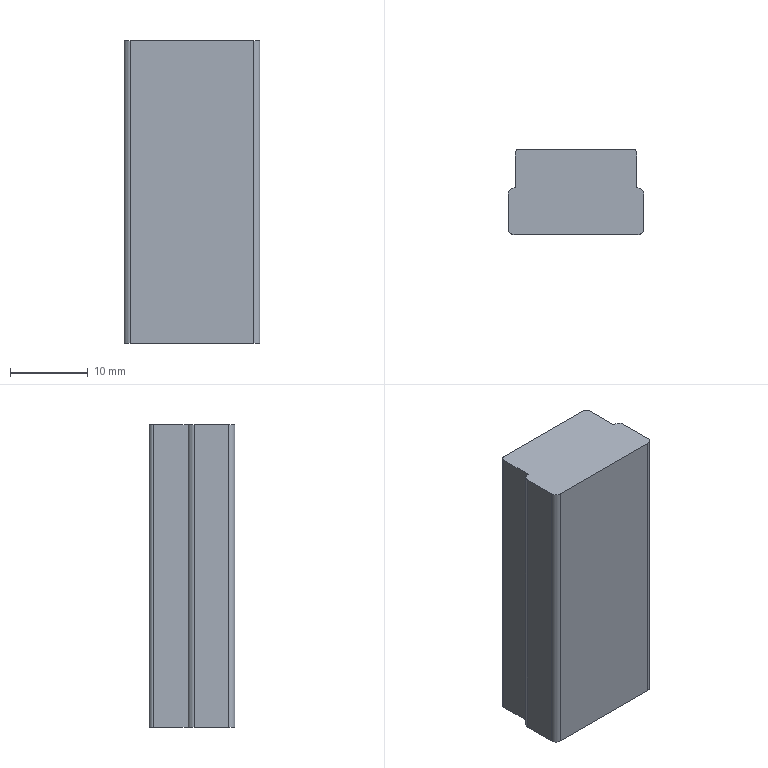Part | STEP file | LUOI GA PHIA DUOI | 1 solid | 16 faces | box 17.5 x 11 x 39 mm | volume 7111 mm3 | plane 10 | cylinder 6 | commonest cylinder face diameters 1.6 x4 1 x2
STEP:
#1=CARTESIAN_POINT('',(0.,0.,0.));
#2=DIRECTION('',(0.,0.,1.));
#3=DIRECTION('',(1.,0.,0.));
#4=AXIS2_PLACEMENT_3D('',#1,#2,#3);
#5=CARTESIAN_POINT('',(-16.7,0.,0.));
#6=VERTEX_POINT('',#5);
#7=CARTESIAN_POINT('',(-0.8,0.,0.));
#8=VERTEX_POINT('',#7);
#9=CARTESIAN_POINT('',(-0.8,0.,0.));
#10=DIRECTION('',(1.,0.,0.));
#11=VECTOR('',#10,1.);
#12=LINE('',#9,#11);
#13=CARTESIAN_POINT('',(-0.8,0.,0.));
#14=DIRECTION('',(0.,-1.,0.));
#15=DIRECTION('',(0.,0.,-1.));
#16=AXIS2_PLACEMENT_3D('',#13,#14,#15);
#17=PLANE('',#16);
#18=CARTESIAN_POINT('',(0.,0.));
#19=DIRECTION('',(0.,1.));
#20=VECTOR('',#19,1.);
#21=LINE('',#18,#20);
#22=(GEOMETRIC_REPRESENTATION_CONTEXT(2)PARAMETRIC_REPRESENTATION_CONTEXT()REPRESENTATION_CONTEXT('',''));
#23=DEFINITIONAL_REPRESENTATION('',(#21),#22);
#24=PCURVE('',#17,#23);
#25=CARTESIAN_POINT('',(-8.75,5.346,0.));
#26=DIRECTION('',(0.,0.,1.));
#27=DIRECTION('',(1.,0.,0.));
#28=AXIS2_PLACEMENT_3D('',#25,#26,#27);
#29=PLANE('',#28);
#30=CARTESIAN_POINT('',(7.95,-5.346));
#31=DIRECTION('',(1.,0.));
#32=VECTOR('',#31,1.);
#33=LINE('',#30,#32);
#34=(GEOMETRIC_REPRESENTATION_CONTEXT(2)PARAMETRIC_REPRESENTATION_CONTEXT()REPRESENTATION_CONTEXT('',''));
#35=DEFINITIONAL_REPRESENTATION('',(#33),#34);
#36=PCURVE('',#29,#35);
#37=SURFACE_CURVE('',#12,(#24,#36),.PCURVE_S1.);
#38=EDGE_CURVE('',#6,#8,#37,.T.);
#39=ORIENTED_EDGE('',*,*,#38,.T.);
#40=CARTESIAN_POINT('',(-0.8,0.,39.));
#41=VERTEX_POINT('',#40);
#42=CARTESIAN_POINT('',(-0.8,0.,0.));
#43=DIRECTION('',(0.,0.,1.));
#44=VECTOR('',#43,1.);
#45=LINE('',#42,#44);
#46=CARTESIAN_POINT('',(0.,0.));
#47=DIRECTION('',(-1.,0.));
#48=VECTOR('',#47,1.);
#49=LINE('',#46,#48);
#50=(GEOMETRIC_REPRESENTATION_CONTEXT(2)PARAMETRIC_REPRESENTATION_CONTEXT()REPRESENTATION_CONTEXT('',''));
#51=DEFINITIONAL_REPRESENTATION('',(#49),#50);
#52=PCURVE('',#17,#51);
#53=CARTESIAN_POINT('',(-0.8,0.8,0.));
#54=DIRECTION('',(0.,0.,1.));
#55=DIRECTION('',(1.,0.,0.));
#56=AXIS2_PLACEMENT_3D('',#53,#54,#55);
#57=CYLINDRICAL_SURFACE('',#56,0.8);
#58=CARTESIAN_POINT('',(4.712,0.));
#59=DIRECTION('',(0.,1.));
#60=VECTOR('',#59,1.);
#61=LINE('',#58,#60);
#62=(GEOMETRIC_REPRESENTATION_CONTEXT(2)PARAMETRIC_REPRESENTATION_CONTEXT()REPRESENTATION_CONTEXT('',''));
#63=DEFINITIONAL_REPRESENTATION('',(#61),#62);
#64=PCURVE('',#57,#63);
#65=SURFACE_CURVE('',#45,(#52,#64),.PCURVE_S1.);
#66=EDGE_CURVE('',#8,#41,#65,.T.);
#67=ORIENTED_EDGE('',*,*,#66,.T.);
#68=CARTESIAN_POINT('',(-16.7,0.,39.));
#69=VERTEX_POINT('',#68);
#70=CARTESIAN_POINT('',(-0.8,0.,39.));
#71=DIRECTION('',(-1.,0.,0.));
#72=VECTOR('',#71,1.);
#73=LINE('',#70,#72);
#74=CARTESIAN_POINT('',(-39.,0.));
#75=DIRECTION('',(0.,-1.));
#76=VECTOR('',#75,1.);
#77=LINE('',#74,#76);
#78=(GEOMETRIC_REPRESENTATION_CONTEXT(2)PARAMETRIC_REPRESENTATION_CONTEXT()REPRESENTATION_CONTEXT('',''));
#79=DEFINITIONAL_REPRESENTATION('',(#77),#78);
#80=PCURVE('',#17,#79);
#81=CARTESIAN_POINT('',(-8.75,5.346,39.));
#82=DIRECTION('',(0.,0.,1.));
#83=DIRECTION('',(1.,0.,0.));
#84=AXIS2_PLACEMENT_3D('',#81,#82,#83);
#85=PLANE('',#84);
#86=CARTESIAN_POINT('',(7.95,-5.346));
#87=DIRECTION('',(-1.,0.));
#88=VECTOR('',#87,1.);
#89=LINE('',#86,#88);
#90=(GEOMETRIC_REPRESENTATION_CONTEXT(2)PARAMETRIC_REPRESENTATION_CONTEXT()REPRESENTATION_CONTEXT('',''));
#91=DEFINITIONAL_REPRESENTATION('',(#89),#90);
#92=PCURVE('',#85,#91);
#93=SURFACE_CURVE('',#73,(#80,#92),.PCURVE_S1.);
#94=EDGE_CURVE('',#41,#69,#93,.T.);
#95=ORIENTED_EDGE('',*,*,#94,.T.);
#96=CARTESIAN_POINT('',(-16.7,0.,0.));
#97=DIRECTION('',(0.,0.,-1.));
#98=VECTOR('',#97,1.);
#99=LINE('',#96,#98);
#100=CARTESIAN_POINT('',(0.,-15.9));
#101=DIRECTION('',(1.,0.));
#102=VECTOR('',#101,1.);
#103=LINE('',#100,#102);
#104=(GEOMETRIC_REPRESENTATION_CONTEXT(2)PARAMETRIC_REPRESENTATION_CONTEXT()REPRESENTATION_CONTEXT('',''));
#105=DEFINITIONAL_REPRESENTATION('',(#103),#104);
#106=PCURVE('',#17,#105);
#107=CARTESIAN_POINT('',(-16.7,0.8,0.));
#108=DIRECTION('',(0.,0.,1.));
#109=DIRECTION('',(1.,0.,0.));
#110=AXIS2_PLACEMENT_3D('',#107,#108,#109);
#111=CYLINDRICAL_SURFACE('',#110,0.8);
#112=CARTESIAN_POINT('',(4.712,0.));
#113=DIRECTION('',(0.,-1.));
#114=VECTOR('',#113,1.);
#115=LINE('',#112,#114);
#116=(GEOMETRIC_REPRESENTATION_CONTEXT(2)PARAMETRIC_REPRESENTATION_CONTEXT()REPRESENTATION_CONTEXT('',''));
#117=DEFINITIONAL_REPRESENTATION('',(#115),#116);
#118=PCURVE('',#111,#117);
#119=SURFACE_CURVE('',#99,(#106,#118),.PCURVE_S1.);
#120=EDGE_CURVE('',#69,#6,#119,.T.);
#121=ORIENTED_EDGE('',*,*,#120,.T.);
#122=EDGE_LOOP('',(#39,#67,#95,#121));
#123=FACE_BOUND('',#122,.T.);
#124=ADVANCED_FACE('',(#123),#17,.T.);
#125=CARTESIAN_POINT('',(0.,0.8,0.));
#126=VERTEX_POINT('',#125);
#127=CARTESIAN_POINT('',(-0.8,0.8,0.));
#128=DIRECTION('',(0.,0.,1.));
#129=DIRECTION('',(1.,0.,0.));
#130=AXIS2_PLACEMENT_3D('',#127,#128,#129);
#131=CIRCLE('',#130,0.8);
#132=CARTESIAN_POINT('',(0.,0.));
#133=DIRECTION('',(1.,0.));
#134=VECTOR('',#133,1.);
#135=LINE('',#132,#134);
#136=(GEOMETRIC_REPRESENTATION_CONTEXT(2)PARAMETRIC_REPRESENTATION_CONTEXT()REPRESENTATION_CONTEXT('',''));
#137=DEFINITIONAL_REPRESENTATION('',(#135),#136);
#138=PCURVE('',#57,#137);
#139=CARTESIAN_POINT('',(7.95,-4.546));
#140=DIRECTION('',(1.,0.));
#141=AXIS2_PLACEMENT_2D('',#139,#140);
#142=CIRCLE('',#141,0.8);
#143=(GEOMETRIC_REPRESENTATION_CONTEXT(2)PARAMETRIC_REPRESENTATION_CONTEXT()REPRESENTATION_CONTEXT('',''));
#144=DEFINITIONAL_REPRESENTATION('',(#142),#143);
#145=PCURVE('',#29,#144);
#146=SURFACE_CURVE('',#131,(#138,#145),.PCURVE_S1.);
#147=EDGE_CURVE('',#8,#126,#146,.T.);
#148=ORIENTED_EDGE('',*,*,#147,.T.);
#149=CARTESIAN_POINT('',(0.,0.8,39.));
#150=VERTEX_POINT('',#149);
#151=CARTESIAN_POINT('',(0.,0.8,0.));
#152=DIRECTION('',(0.,0.,1.));
#153=VECTOR('',#152,1.);
#154=LINE('',#151,#153);
#155=CARTESIAN_POINT('',(6.283,0.));
#156=DIRECTION('',(0.,1.));
#157=VECTOR('',#156,1.);
#158=LINE('',#155,#157);
#159=(GEOMETRIC_REPRESENTATION_CONTEXT(2)PARAMETRIC_REPRESENTATION_CONTEXT()REPRESENTATION_CONTEXT('',''));
#160=DEFINITIONAL_REPRESENTATION('',(#158),#159);
#161=PCURVE('',#57,#160);
#162=CARTESIAN_POINT('',(0.,5.2,0.));
#163=DIRECTION('',(1.,0.,0.));
#164=DIRECTION('',(0.,0.,-1.));
#165=AXIS2_PLACEMENT_3D('',#162,#163,#164);
#166=PLANE('',#165);
#167=CARTESIAN_POINT('',(0.,-4.4));
#168=DIRECTION('',(-1.,0.));
#169=VECTOR('',#168,1.);
#170=LINE('',#167,#169);
#171=(GEOMETRIC_REPRESENTATION_CONTEXT(2)PARAMETRIC_REPRESENTATION_CONTEXT()REPRESENTATION_CONTEXT('',''));
#172=DEFINITIONAL_REPRESENTATION('',(#170),#171);
#173=PCURVE('',#166,#172);
#174=SURFACE_CURVE('',#154,(#161,#173),.PCURVE_S1.);
#175=EDGE_CURVE('',#126,#150,#174,.T.);
#176=ORIENTED_EDGE('',*,*,#175,.T.);
#177=CARTESIAN_POINT('',(-0.8,0.8,39.));
#178=DIRECTION('',(0.,0.,-1.));
#179=DIRECTION('',(1.,0.,0.));
#180=AXIS2_PLACEMENT_3D('',#177,#178,#179);
#181=CIRCLE('',#180,0.8);
#182=CARTESIAN_POINT('',(6.283,39.));
#183=DIRECTION('',(-1.,0.));
#184=VECTOR('',#183,1.);
#185=LINE('',#182,#184);
#186=(GEOMETRIC_REPRESENTATION_CONTEXT(2)PARAMETRIC_REPRESENTATION_CONTEXT()REPRESENTATION_CONTEXT('',''));
#187=DEFINITIONAL_REPRESENTATION('',(#185),#186);
#188=PCURVE('',#57,#187);
#189=CARTESIAN_POINT('',(8.75,-4.546));
#190=CARTESIAN_POINT('',(8.75,-5.932));
#191=CARTESIAN_POINT('',(7.55,-5.239));
#192=CARTESIAN_POINT('',(6.35,-4.546));
#193=CARTESIAN_POINT('',(7.55,-3.854));
#194=CARTESIAN_POINT('',(8.75,-3.161));
#195=CARTESIAN_POINT('',(8.75,-4.546));
#196=(BOUNDED_CURVE()B_SPLINE_CURVE(2,(#189,#190,#191,#192,#193,#194,#195),.UNSPECIFIED.,.T.,.F.)B_SPLINE_CURVE_WITH_KNOTS((1,2,2,2,2,1),(-2.094,0.,2.094,4.189,6.283,8.378),.UNSPECIFIED.)CURVE()GEOMETRIC_REPRESENTATION_ITEM()RATIONAL_B_SPLINE_CURVE((1.,0.5,1.,0.5,1.,0.5,1.))REPRESENTATION_ITEM(''));
#197=(GEOMETRIC_REPRESENTATION_CONTEXT(2)PARAMETRIC_REPRESENTATION_CONTEXT()REPRESENTATION_CONTEXT('',''));
#198=DEFINITIONAL_REPRESENTATION('',(#196),#197);
#199=PCURVE('',#85,#198);
#200=SURFACE_CURVE('',#181,(#188,#199),.PCURVE_S1.);
#201=EDGE_CURVE('',#150,#41,#200,.T.);
#202=ORIENTED_EDGE('',*,*,#201,.T.);
#203=ORIENTED_EDGE('',*,*,#66,.F.);
#204=EDGE_LOOP('',(#148,#176,#202,#203));
#205=FACE_BOUND('',#204,.T.);
#206=ADVANCED_FACE('',(#205),#57,.T.);
#207=CARTESIAN_POINT('',(-0.8,6.,0.));
#208=VERTEX_POINT('',#207);
#209=CARTESIAN_POINT('',(-0.95,6.,0.));
#210=VERTEX_POINT('',#209);
#211=CARTESIAN_POINT('',(-0.95,6.,0.));
#212=DIRECTION('',(-1.,0.,0.));
#213=VECTOR('',#212,1.);
#214=LINE('',#211,#213);
#215=CARTESIAN_POINT('',(7.8,0.6535));
#216=DIRECTION('',(-1.,0.));
#217=VECTOR('',#216,1.);
#218=LINE('',#215,#217);
#219=(GEOMETRIC_REPRESENTATION_CONTEXT(2)PARAMETRIC_REPRESENTATION_CONTEXT()REPRESENTATION_CONTEXT('',''));
#220=DEFINITIONAL_REPRESENTATION('',(#218),#219);
#221=PCURVE('',#29,#220);
#222=CARTESIAN_POINT('',(-0.95,6.,0.));
#223=DIRECTION('',(0.,1.,0.));
#224=DIRECTION('',(0.,0.,1.));
#225=AXIS2_PLACEMENT_3D('',#222,#223,#224);
#226=PLANE('',#225);
#227=CARTESIAN_POINT('',(0.,0.));
#228=DIRECTION('',(0.,-1.));
#229=VECTOR('',#228,1.);
#230=LINE('',#227,#229);
#231=(GEOMETRIC_REPRESENTATION_CONTEXT(2)PARAMETRIC_REPRESENTATION_CONTEXT()REPRESENTATION_CONTEXT('',''));
#232=DEFINITIONAL_REPRESENTATION('',(#230),#231);
#233=PCURVE('',#226,#232);
#234=SURFACE_CURVE('',#214,(#221,#233),.PCURVE_S1.);
#235=EDGE_CURVE('',#208,#210,#234,.T.);
#236=ORIENTED_EDGE('',*,*,#235,.F.);
#237=CARTESIAN_POINT('',(0.,5.2,0.));
#238=VERTEX_POINT('',#237);
#239=CARTESIAN_POINT('',(-0.8,5.2,0.));
#240=DIRECTION('',(0.,0.,1.));
#241=DIRECTION('',(1.,0.,0.));
#242=AXIS2_PLACEMENT_3D('',#239,#240,#241);
#243=CIRCLE('',#242,0.8);
#244=CARTESIAN_POINT('',(7.95,-0.1465));
#245=DIRECTION('',(1.,0.));
#246=AXIS2_PLACEMENT_2D('',#244,#245);
#247=CIRCLE('',#246,0.8);
#248=(GEOMETRIC_REPRESENTATION_CONTEXT(2)PARAMETRIC_REPRESENTATION_CONTEXT()REPRESENTATION_CONTEXT('',''));
#249=DEFINITIONAL_REPRESENTATION('',(#247),#248);
#250=PCURVE('',#29,#249);
#251=CARTESIAN_POINT('',(-0.8,5.2,0.));
#252=DIRECTION('',(0.,0.,1.));
#253=DIRECTION('',(1.,0.,0.));
#254=AXIS2_PLACEMENT_3D('',#251,#252,#253);
#255=CYLINDRICAL_SURFACE('',#254,0.8);
#256=CARTESIAN_POINT('',(0.,0.));
#257=DIRECTION('',(1.,0.));
#258=VECTOR('',#257,1.);
#259=LINE('',#256,#258);
#260=(GEOMETRIC_REPRESENTATION_CONTEXT(2)PARAMETRIC_REPRESENTATION_CONTEXT()REPRESENTATION_CONTEXT('',''));
#261=DEFINITIONAL_REPRESENTATION('',(#259),#260);
#262=PCURVE('',#255,#261);
#263=SURFACE_CURVE('',#243,(#250,#262),.PCURVE_S1.);
#264=EDGE_CURVE('',#238,#208,#263,.T.);
#265=ORIENTED_EDGE('',*,*,#264,.F.);
#266=CARTESIAN_POINT('',(0.,5.346,0.));
#267=DIRECTION('',(0.,1.,0.));
#268=VECTOR('',#267,1.);
#269=LINE('',#266,#268);
#270=CARTESIAN_POINT('',(8.75,0.));
#271=DIRECTION('',(0.,1.));
#272=VECTOR('',#271,1.);
#273=LINE('',#270,#272);
#274=(GEOMETRIC_REPRESENTATION_CONTEXT(2)PARAMETRIC_REPRESENTATION_CONTEXT()REPRESENTATION_CONTEXT('',''));
#275=DEFINITIONAL_REPRESENTATION('',(#273),#274);
#276=PCURVE('',#29,#275);
#277=CARTESIAN_POINT('',(0.,0.1465));
#278=DIRECTION('',(0.,1.));
#279=VECTOR('',#278,1.);
#280=LINE('',#277,#279);
#281=(GEOMETRIC_REPRESENTATION_CONTEXT(2)PARAMETRIC_REPRESENTATION_CONTEXT()REPRESENTATION_CONTEXT('',''));
#282=DEFINITIONAL_REPRESENTATION('',(#280),#281);
#283=PCURVE('',#166,#282);
#284=SURFACE_CURVE('',#269,(#276,#283),.PCURVE_S1.);
#285=EDGE_CURVE('',#126,#238,#284,.T.);
#286=ORIENTED_EDGE('',*,*,#285,.F.);
#287=ORIENTED_EDGE('',*,*,#147,.F.);
#288=ORIENTED_EDGE('',*,*,#38,.F.);
#289=CARTESIAN_POINT('',(-17.5,0.8,0.));
#290=VERTEX_POINT('',#289);
#291=CARTESIAN_POINT('',(-16.7,0.8,0.));
#292=DIRECTION('',(0.,0.,1.));
#293=DIRECTION('',(1.,0.,0.));
#294=AXIS2_PLACEMENT_3D('',#291,#292,#293);
#295=CIRCLE('',#294,0.8);
#296=CARTESIAN_POINT('',(-7.95,-4.546));
#297=DIRECTION('',(1.,0.));
#298=AXIS2_PLACEMENT_2D('',#296,#297);
#299=CIRCLE('',#298,0.8);
#300=(GEOMETRIC_REPRESENTATION_CONTEXT(2)PARAMETRIC_REPRESENTATION_CONTEXT()REPRESENTATION_CONTEXT('',''));
#301=DEFINITIONAL_REPRESENTATION('',(#299),#300);
#302=PCURVE('',#29,#301);
#303=CARTESIAN_POINT('',(0.,0.));
#304=DIRECTION('',(1.,0.));
#305=VECTOR('',#304,1.);
#306=LINE('',#303,#305);
#307=(GEOMETRIC_REPRESENTATION_CONTEXT(2)PARAMETRIC_REPRESENTATION_CONTEXT()REPRESENTATION_CONTEXT('',''));
#308=DEFINITIONAL_REPRESENTATION('',(#306),#307);
#309=PCURVE('',#111,#308);
#310=SURFACE_CURVE('',#295,(#302,#309),.PCURVE_S1.);
#311=EDGE_CURVE('',#290,#6,#310,.T.);
#312=ORIENTED_EDGE('',*,*,#311,.F.);
#313=CARTESIAN_POINT('',(-17.5,5.2,0.));
#314=VERTEX_POINT('',#313);
#315=CARTESIAN_POINT('',(-17.5,5.346,0.));
#316=DIRECTION('',(0.,-1.,0.));
#317=VECTOR('',#316,1.);
#318=LINE('',#315,#317);
#319=CARTESIAN_POINT('',(-8.75,0.));
#320=DIRECTION('',(0.,-1.));
#321=VECTOR('',#320,1.);
#322=LINE('',#319,#321);
#323=(GEOMETRIC_REPRESENTATION_CONTEXT(2)PARAMETRIC_REPRESENTATION_CONTEXT()REPRESENTATION_CONTEXT('',''));
#324=DEFINITIONAL_REPRESENTATION('',(#322),#323);
#325=PCURVE('',#29,#324);
#326=CARTESIAN_POINT('',(-17.5,0.8,0.));
#327=DIRECTION('',(-1.,0.,0.));
#328=DIRECTION('',(0.,0.,1.));
#329=AXIS2_PLACEMENT_3D('',#326,#327,#328);
#330=PLANE('',#329);
#331=CARTESIAN_POINT('',(0.,4.546));
#332=DIRECTION('',(0.,-1.));
#333=VECTOR('',#332,1.);
#334=LINE('',#331,#333);
#335=(GEOMETRIC_REPRESENTATION_CONTEXT(2)PARAMETRIC_REPRESENTATION_CONTEXT()REPRESENTATION_CONTEXT('',''));
#336=DEFINITIONAL_REPRESENTATION('',(#334),#335);
#337=PCURVE('',#330,#336);
#338=SURFACE_CURVE('',#318,(#325,#337),.PCURVE_S1.);
#339=EDGE_CURVE('',#314,#290,#338,.T.);
#340=ORIENTED_EDGE('',*,*,#339,.F.);
#341=CARTESIAN_POINT('',(-16.7,6.,0.));
#342=VERTEX_POINT('',#341);
#343=CARTESIAN_POINT('',(-16.7,5.2,0.));
#344=DIRECTION('',(0.,0.,1.));
#345=DIRECTION('',(1.,0.,0.));
#346=AXIS2_PLACEMENT_3D('',#343,#344,#345);
#347=CIRCLE('',#346,0.8);
#348=CARTESIAN_POINT('',(-7.95,-0.1465));
#349=DIRECTION('',(1.,0.));
#350=AXIS2_PLACEMENT_2D('',#348,#349);
#351=CIRCLE('',#350,0.8);
#352=(GEOMETRIC_REPRESENTATION_CONTEXT(2)PARAMETRIC_REPRESENTATION_CONTEXT()REPRESENTATION_CONTEXT('',''));
#353=DEFINITIONAL_REPRESENTATION('',(#351),#352);
#354=PCURVE('',#29,#353);
#355=CARTESIAN_POINT('',(-16.7,5.2,0.));
#356=DIRECTION('',(0.,0.,1.));
#357=DIRECTION('',(1.,0.,0.));
#358=AXIS2_PLACEMENT_3D('',#355,#356,#357);
#359=CYLINDRICAL_SURFACE('',#358,0.8);
#360=CARTESIAN_POINT('',(0.,0.));
#361=DIRECTION('',(1.,0.));
#362=VECTOR('',#361,1.);
#363=LINE('',#360,#362);
#364=(GEOMETRIC_REPRESENTATION_CONTEXT(2)PARAMETRIC_REPRESENTATION_CONTEXT()REPRESENTATION_CONTEXT('',''));
#365=DEFINITIONAL_REPRESENTATION('',(#363),#364);
#366=PCURVE('',#359,#365);
#367=SURFACE_CURVE('',#347,(#354,#366),.PCURVE_S1.);
#368=EDGE_CURVE('',#342,#314,#367,.T.);
#369=ORIENTED_EDGE('',*,*,#368,.F.);
#370=CARTESIAN_POINT('',(-16.55,6.,0.));
#371=VERTEX_POINT('',#370);
#372=CARTESIAN_POINT('',(-16.7,6.,0.));
#373=DIRECTION('',(-1.,0.,0.));
#374=VECTOR('',#373,1.);
#375=LINE('',#372,#374);
#376=CARTESIAN_POINT('',(-7.95,0.6535));
#377=DIRECTION('',(-1.,0.));
#378=VECTOR('',#377,1.);
#379=LINE('',#376,#378);
#380=(GEOMETRIC_REPRESENTATION_CONTEXT(2)PARAMETRIC_REPRESENTATION_CONTEXT()REPRESENTATION_CONTEXT('',''));
#381=DEFINITIONAL_REPRESENTATION('',(#379),#380);
#382=PCURVE('',#29,#381);
#383=CARTESIAN_POINT('',(-16.7,6.,0.));
#384=DIRECTION('',(0.,1.,0.));
#385=DIRECTION('',(0.,0.,1.));
#386=AXIS2_PLACEMENT_3D('',#383,#384,#385);
#387=PLANE('',#386);
#388=CARTESIAN_POINT('',(0.,0.));
#389=DIRECTION('',(0.,-1.));
#390=VECTOR('',#389,1.);
#391=LINE('',#388,#390);
#392=(GEOMETRIC_REPRESENTATION_CONTEXT(2)PARAMETRIC_REPRESENTATION_CONTEXT()REPRESENTATION_CONTEXT('',''));
#393=DEFINITIONAL_REPRESENTATION('',(#391),#392);
#394=PCURVE('',#387,#393);
#395=SURFACE_CURVE('',#375,(#382,#394),.PCURVE_S1.);
#396=EDGE_CURVE('',#371,#342,#395,.T.);
#397=ORIENTED_EDGE('',*,*,#396,.F.);
#398=CARTESIAN_POINT('',(-16.55,10.5,0.));
#399=VERTEX_POINT('',#398);
#400=CARTESIAN_POINT('',(-16.55,5.346,0.));
#401=DIRECTION('',(0.,-1.,0.));
#402=VECTOR('',#401,1.);
#403=LINE('',#400,#402);
#404=CARTESIAN_POINT('',(-7.8,0.));
#405=DIRECTION('',(0.,-1.));
#406=VECTOR('',#405,1.);
#407=LINE('',#404,#406);
#408=(GEOMETRIC_REPRESENTATION_CONTEXT(2)PARAMETRIC_REPRESENTATION_CONTEXT()REPRESENTATION_CONTEXT('',''));
#409=DEFINITIONAL_REPRESENTATION('',(#407),#408);
#410=PCURVE('',#29,#409);
#411=CARTESIAN_POINT('',(-16.55,6.,0.));
#412=DIRECTION('',(-1.,0.,0.));
#413=DIRECTION('',(0.,0.,1.));
#414=AXIS2_PLACEMENT_3D('',#411,#412,#413);
#415=PLANE('',#414);
#416=CARTESIAN_POINT('',(0.,-0.6535));
#417=DIRECTION('',(0.,-1.));
#418=VECTOR('',#417,1.);
#419=LINE('',#416,#418);
#420=(GEOMETRIC_REPRESENTATION_CONTEXT(2)PARAMETRIC_REPRESENTATION_CONTEXT()REPRESENTATION_CONTEXT('',''));
#421=DEFINITIONAL_REPRESENTATION('',(#419),#420);
#422=PCURVE('',#415,#421);
#423=SURFACE_CURVE('',#403,(#410,#422),.PCURVE_S1.);
#424=EDGE_CURVE('',#399,#371,#423,.T.);
#425=ORIENTED_EDGE('',*,*,#424,.F.);
#426=CARTESIAN_POINT('',(-16.05,11.,0.));
#427=VERTEX_POINT('',#426);
#428=CARTESIAN_POINT('',(-16.05,10.5,0.));
#429=DIRECTION('',(0.,0.,1.));
#430=DIRECTION('',(1.,0.,0.));
#431=AXIS2_PLACEMENT_3D('',#428,#429,#430);
#432=CIRCLE('',#431,0.5);
#433=CARTESIAN_POINT('',(-7.3,5.154));
#434=DIRECTION('',(1.,0.));
#435=AXIS2_PLACEMENT_2D('',#433,#434);
#436=CIRCLE('',#435,0.5);
#437=(GEOMETRIC_REPRESENTATION_CONTEXT(2)PARAMETRIC_REPRESENTATION_CONTEXT()REPRESENTATION_CONTEXT('',''));
#438=DEFINITIONAL_REPRESENTATION('',(#436),#437);
#439=PCURVE('',#29,#438);
#440=CARTESIAN_POINT('',(-16.05,10.5,0.));
#441=DIRECTION('',(0.,0.,1.));
#442=DIRECTION('',(1.,0.,0.));
#443=AXIS2_PLACEMENT_3D('',#440,#441,#442);
#444=CYLINDRICAL_SURFACE('',#443,0.5);
#445=CARTESIAN_POINT('',(0.,0.));
#446=DIRECTION('',(1.,0.));
#447=VECTOR('',#446,1.);
#448=LINE('',#445,#447);
#449=(GEOMETRIC_REPRESENTATION_CONTEXT(2)PARAMETRIC_REPRESENTATION_CONTEXT()REPRESENTATION_CONTEXT('',''));
#450=DEFINITIONAL_REPRESENTATION('',(#448),#449);
#451=PCURVE('',#444,#450);
#452=SURFACE_CURVE('',#432,(#439,#451),.PCURVE_S1.);
#453=EDGE_CURVE('',#427,#399,#452,.T.);
#454=ORIENTED_EDGE('',*,*,#453,.F.);
#455=CARTESIAN_POINT('',(-1.45,11.,0.));
#456=VERTEX_POINT('',#455);
#457=CARTESIAN_POINT('',(-8.75,11.,0.));
#458=DIRECTION('',(-1.,0.,0.));
#459=VECTOR('',#458,1.);
#460=LINE('',#457,#459);
#461=CARTESIAN_POINT('',(0.,5.654));
#462=DIRECTION('',(-1.,0.));
#463=VECTOR('',#462,1.);
#464=LINE('',#461,#463);
#465=(GEOMETRIC_REPRESENTATION_CONTEXT(2)PARAMETRIC_REPRESENTATION_CONTEXT()REPRESENTATION_CONTEXT('',''));
#466=DEFINITIONAL_REPRESENTATION('',(#464),#465);
#467=PCURVE('',#29,#466);
#468=CARTESIAN_POINT('',(-16.05,11.,0.));
#469=DIRECTION('',(0.,1.,0.));
#470=DIRECTION('',(0.,0.,1.));
#471=AXIS2_PLACEMENT_3D('',#468,#469,#470);
#472=PLANE('',#471);
#473=CARTESIAN_POINT('',(0.,7.3));
#474=DIRECTION('',(0.,-1.));
#475=VECTOR('',#474,1.);
#476=LINE('',#473,#475);
#477=(GEOMETRIC_REPRESENTATION_CONTEXT(2)PARAMETRIC_REPRESENTATION_CONTEXT()REPRESENTATION_CONTEXT('',''));
#478=DEFINITIONAL_REPRESENTATION('',(#476),#477);
#479=PCURVE('',#472,#478);
#480=SURFACE_CURVE('',#460,(#467,#479),.PCURVE_S1.);
#481=EDGE_CURVE('',#456,#427,#480,.T.);
#482=ORIENTED_EDGE('',*,*,#481,.F.);
#483=CARTESIAN_POINT('',(-0.95,10.5,0.));
#484=VERTEX_POINT('',#483);
#485=CARTESIAN_POINT('',(-1.45,10.5,0.));
#486=DIRECTION('',(0.,0.,1.));
#487=DIRECTION('',(1.,0.,0.));
#488=AXIS2_PLACEMENT_3D('',#485,#486,#487);
#489=CIRCLE('',#488,0.5);
#490=CARTESIAN_POINT('',(7.3,5.154));
#491=DIRECTION('',(1.,0.));
#492=AXIS2_PLACEMENT_2D('',#490,#491);
#493=CIRCLE('',#492,0.5);
#494=(GEOMETRIC_REPRESENTATION_CONTEXT(2)PARAMETRIC_REPRESENTATION_CONTEXT()REPRESENTATION_CONTEXT('',''));
#495=DEFINITIONAL_REPRESENTATION('',(#493),#494);
#496=PCURVE('',#29,#495);
#497=CARTESIAN_POINT('',(-1.45,10.5,0.));
#498=DIRECTION('',(0.,0.,1.));
#499=DIRECTION('',(1.,0.,0.));
#500=AXIS2_PLACEMENT_3D('',#497,#498,#499);
#501=CYLINDRICAL_SURFACE('',#500,0.5);
#502=CARTESIAN_POINT('',(0.,0.));
#503=DIRECTION('',(1.,0.));
#504=VECTOR('',#503,1.);
#505=LINE('',#502,#504);
#506=(GEOMETRIC_REPRESENTATION_CONTEXT(2)PARAMETRIC_REPRESENTATION_CONTEXT()REPRESENTATION_CONTEXT('',''));
#507=DEFINITIONAL_REPRESENTATION('',(#505),#506);
#508=PCURVE('',#501,#507);
#509=SURFACE_CURVE('',#489,(#496,#508),.PCURVE_S1.);
#510=EDGE_CURVE('',#484,#456,#509,.T.);
#511=ORIENTED_EDGE('',*,*,#510,.F.);
#512=CARTESIAN_POINT('',(-0.95,5.346,0.));
#513=DIRECTION('',(0.,1.,0.));
#514=VECTOR('',#513,1.);
#515=LINE('',#512,#514);
#516=CARTESIAN_POINT('',(7.8,0.));
#517=DIRECTION('',(0.,1.));
#518=VECTOR('',#517,1.);
#519=LINE('',#516,#518);
#520=(GEOMETRIC_REPRESENTATION_CONTEXT(2)PARAMETRIC_REPRESENTATION_CONTEXT()REPRESENTATION_CONTEXT('',''));
#521=DEFINITIONAL_REPRESENTATION('',(#519),#520);
#522=PCURVE('',#29,#521);
#523=CARTESIAN_POINT('',(-0.95,10.5,0.));
#524=DIRECTION('',(1.,0.,0.));
#525=DIRECTION('',(0.,0.,-1.));
#526=AXIS2_PLACEMENT_3D('',#523,#524,#525);
#527=PLANE('',#526);
#528=CARTESIAN_POINT('',(0.,-5.154));
#529=DIRECTION('',(0.,1.));
#530=VECTOR('',#529,1.);
#531=LINE('',#528,#530);
#532=(GEOMETRIC_REPRESENTATION_CONTEXT(2)PARAMETRIC_REPRESENTATION_CONTEXT()REPRESENTATION_CONTEXT('',''));
#533=DEFINITIONAL_REPRESENTATION('',(#531),#532);
#534=PCURVE('',#527,#533);
#535=SURFACE_CURVE('',#515,(#522,#534),.PCURVE_S1.);
#536=EDGE_CURVE('',#210,#484,#535,.T.);
#537=ORIENTED_EDGE('',*,*,#536,.F.);
#538=EDGE_LOOP('',(#236,#265,#286,#287,#288,#312,#340,#369,#397,#425,#454,#482,#511,#537));
#539=FACE_BOUND('',#538,.T.);
#540=ADVANCED_FACE('',(#539),#29,.F.);
#541=ORIENTED_EDGE('',*,*,#311,.T.);
#542=ORIENTED_EDGE('',*,*,#120,.F.);
#543=CARTESIAN_POINT('',(-17.5,0.8,39.));
#544=VERTEX_POINT('',#543);
#545=CARTESIAN_POINT('',(-16.7,0.8,39.));
#546=DIRECTION('',(0.,0.,-1.));
#547=DIRECTION('',(1.,0.,0.));
#548=AXIS2_PLACEMENT_3D('',#545,#546,#547);
#549=CIRCLE('',#548,0.8);
#550=CARTESIAN_POINT('',(6.283,39.));
#551=DIRECTION('',(-1.,0.));
#552=VECTOR('',#551,1.);
#553=LINE('',#550,#552);
#554=(GEOMETRIC_REPRESENTATION_CONTEXT(2)PARAMETRIC_REPRESENTATION_CONTEXT()REPRESENTATION_CONTEXT('',''));
#555=DEFINITIONAL_REPRESENTATION('',(#553),#554);
#556=PCURVE('',#111,#555);
#557=CARTESIAN_POINT('',(-7.15,-4.546));
#558=CARTESIAN_POINT('',(-7.15,-5.932));
#559=CARTESIAN_POINT('',(-8.35,-5.239));
#560=CARTESIAN_POINT('',(-9.55,-4.546));
#561=CARTESIAN_POINT('',(-8.35,-3.854));
#562=CARTESIAN_POINT('',(-7.15,-3.161));
#563=CARTESIAN_POINT('',(-7.15,-4.546));
#564=(BOUNDED_CURVE()B_SPLINE_CURVE(2,(#557,#558,#559,#560,#561,#562,#563),.UNSPECIFIED.,.T.,.F.)B_SPLINE_CURVE_WITH_KNOTS((1,2,2,2,2,1),(-2.094,0.,2.094,4.189,6.283,8.378),.UNSPECIFIED.)CURVE()GEOMETRIC_REPRESENTATION_ITEM()RATIONAL_B_SPLINE_CURVE((1.,0.5,1.,0.5,1.,0.5,1.))REPRESENTATION_ITEM(''));
#565=(GEOMETRIC_REPRESENTATION_CONTEXT(2)PARAMETRIC_REPRESENTATION_CONTEXT()REPRESENTATION_CONTEXT('',''));
#566=DEFINITIONAL_REPRESENTATION('',(#564),#565);
#567=PCURVE('',#85,#566);
#568=SURFACE_CURVE('',#549,(#556,#567),.PCURVE_S1.);
#569=EDGE_CURVE('',#69,#544,#568,.T.);
#570=ORIENTED_EDGE('',*,*,#569,.T.);
#571=CARTESIAN_POINT('',(-17.5,0.8,0.));
#572=DIRECTION('',(0.,0.,-1.));
#573=VECTOR('',#572,1.);
#574=LINE('',#571,#573);
#575=CARTESIAN_POINT('',(3.142,0.));
#576=DIRECTION('',(0.,-1.));
#577=VECTOR('',#576,1.);
#578=LINE('',#575,#577);
#579=(GEOMETRIC_REPRESENTATION_CONTEXT(2)PARAMETRIC_REPRESENTATION_CONTEXT()REPRESENTATION_CONTEXT('',''));
#580=DEFINITIONAL_REPRESENTATION('',(#578),#579);
#581=PCURVE('',#111,#580);
#582=CARTESIAN_POINT('',(0.,0.));
#583=DIRECTION('',(-1.,0.));
#584=VECTOR('',#583,1.);
#585=LINE('',#582,#584);
#586=(GEOMETRIC_REPRESENTATION_CONTEXT(2)PARAMETRIC_REPRESENTATION_CONTEXT()REPRESENTATION_CONTEXT('',''));
#587=DEFINITIONAL_REPRESENTATION('',(#585),#586);
#588=PCURVE('',#330,#587);
#589=SURFACE_CURVE('',#574,(#581,#588),.PCURVE_S1.);
#590=EDGE_CURVE('',#544,#290,#589,.T.);
#591=ORIENTED_EDGE('',*,*,#590,.T.);
#592=EDGE_LOOP('',(#541,#542,#570,#591));
#593=FACE_BOUND('',#592,.T.);
#594=ADVANCED_FACE('',(#593),#111,.T.);
#595=CARTESIAN_POINT('',(0.,5.2,39.));
#596=VERTEX_POINT('',#595);
#597=CARTESIAN_POINT('',(0.,5.346,39.));
#598=DIRECTION('',(0.,1.,0.));
#599=VECTOR('',#598,1.);
#600=LINE('',#597,#599);
#601=CARTESIAN_POINT('',(8.75,0.));
#602=DIRECTION('',(0.,1.));
#603=VECTOR('',#602,1.);
#604=LINE('',#601,#603);
#605=(GEOMETRIC_REPRESENTATION_CONTEXT(2)PARAMETRIC_REPRESENTATION_CONTEXT()REPRESENTATION_CONTEXT('',''));
#606=DEFINITIONAL_REPRESENTATION('',(#604),#605);
#607=PCURVE('',#85,#606);
#608=CARTESIAN_POINT('',(-39.,0.1465));
#609=DIRECTION('',(0.,1.));
#610=VECTOR('',#609,1.);
#611=LINE('',#608,#610);
#612=(GEOMETRIC_REPRESENTATION_CONTEXT(2)PARAMETRIC_REPRESENTATION_CONTEXT()REPRESENTATION_CONTEXT('',''));
#613=DEFINITIONAL_REPRESENTATION('',(#611),#612);
#614=PCURVE('',#166,#613);
#615=SURFACE_CURVE('',#600,(#607,#614),.PCURVE_S1.);
#616=EDGE_CURVE('',#150,#596,#615,.T.);
#617=ORIENTED_EDGE('',*,*,#616,.T.);
#618=CARTESIAN_POINT('',(-0.8,6.,39.));
#619=VERTEX_POINT('',#618);
#620=CARTESIAN_POINT('',(-0.8,5.2,39.));
#621=DIRECTION('',(0.,0.,-1.));
#622=DIRECTION('',(1.,0.,0.));
#623=AXIS2_PLACEMENT_3D('',#620,#621,#622);
#624=CIRCLE('',#623,0.8);
#625=CARTESIAN_POINT('',(8.75,-0.1465));
#626=CARTESIAN_POINT('',(8.75,-1.532));
#627=CARTESIAN_POINT('',(7.55,-0.8393));
#628=CARTESIAN_POINT('',(6.35,-0.1465));
#629=CARTESIAN_POINT('',(7.55,0.5463));
#630=CARTESIAN_POINT('',(8.75,1.239));
#631=CARTESIAN_POINT('',(8.75,-0.1465));
#632=(BOUNDED_CURVE()B_SPLINE_CURVE(2,(#625,#626,#627,#628,#629,#630,#631),.UNSPECIFIED.,.T.,.F.)B_SPLINE_CURVE_WITH_KNOTS((1,2,2,2,2,1),(-2.094,0.,2.094,4.189,6.283,8.378),.UNSPECIFIED.)CURVE()GEOMETRIC_REPRESENTATION_ITEM()RATIONAL_B_SPLINE_CURVE((1.,0.5,1.,0.5,1.,0.5,1.))REPRESENTATION_ITEM(''));
#633=(GEOMETRIC_REPRESENTATION_CONTEXT(2)PARAMETRIC_REPRESENTATION_CONTEXT()REPRESENTATION_CONTEXT('',''));
#634=DEFINITIONAL_REPRESENTATION('',(#632),#633);
#635=PCURVE('',#85,#634);
#636=CARTESIAN_POINT('',(6.283,39.));
#637=DIRECTION('',(-1.,0.));
#638=VECTOR('',#637,1.);
#639=LINE('',#636,#638);
#640=(GEOMETRIC_REPRESENTATION_CONTEXT(2)PARAMETRIC_REPRESENTATION_CONTEXT()REPRESENTATION_CONTEXT('',''));
#641=DEFINITIONAL_REPRESENTATION('',(#639),#640);
#642=PCURVE('',#255,#641);
#643=SURFACE_CURVE('',#624,(#635,#642),.PCURVE_S1.);
#644=EDGE_CURVE('',#619,#596,#643,.T.);
#645=ORIENTED_EDGE('',*,*,#644,.F.);
#646=CARTESIAN_POINT('',(-0.95,6.,39.));
#647=VERTEX_POINT('',#646);
#648=CARTESIAN_POINT('',(-0.95,6.,39.));
#649=DIRECTION('',(1.,0.,0.));
#650=VECTOR('',#649,1.);
#651=LINE('',#648,#650);
#652=CARTESIAN_POINT('',(7.8,0.6535));
#653=DIRECTION('',(1.,0.));
#654=VECTOR('',#653,1.);
#655=LINE('',#652,#654);
#656=(GEOMETRIC_REPRESENTATION_CONTEXT(2)PARAMETRIC_REPRESENTATION_CONTEXT()REPRESENTATION_CONTEXT('',''));
#657=DEFINITIONAL_REPRESENTATION('',(#655),#656);
#658=PCURVE('',#85,#657);
#659=CARTESIAN_POINT('',(39.,0.));
#660=DIRECTION('',(0.,1.));
#661=VECTOR('',#660,1.);
#662=LINE('',#659,#661);
#663=(GEOMETRIC_REPRESENTATION_CONTEXT(2)PARAMETRIC_REPRESENTATION_CONTEXT()REPRESENTATION_CONTEXT('',''));
#664=DEFINITIONAL_REPRESENTATION('',(#662),#663);
#665=PCURVE('',#226,#664);
#666=SURFACE_CURVE('',#651,(#658,#665),.PCURVE_S1.);
#667=EDGE_CURVE('',#647,#619,#666,.T.);
#668=ORIENTED_EDGE('',*,*,#667,.F.);
#669=CARTESIAN_POINT('',(-0.95,10.5,39.));
#670=VERTEX_POINT('',#669);
#671=CARTESIAN_POINT('',(-0.95,5.346,39.));
#672=DIRECTION('',(0.,1.,0.));
#673=VECTOR('',#672,1.);
#674=LINE('',#671,#673);
#675=CARTESIAN_POINT('',(7.8,0.));
#676=DIRECTION('',(0.,1.));
#677=VECTOR('',#676,1.);
#678=LINE('',#675,#677);
#679=(GEOMETRIC_REPRESENTATION_CONTEXT(2)PARAMETRIC_REPRESENTATION_CONTEXT()REPRESENTATION_CONTEXT('',''));
#680=DEFINITIONAL_REPRESENTATION('',(#678),#679);
#681=PCURVE('',#85,#680);
#682=CARTESIAN_POINT('',(-39.,-5.154));
#683=DIRECTION('',(0.,1.));
#684=VECTOR('',#683,1.);
#685=LINE('',#682,#684);
#686=(GEOMETRIC_REPRESENTATION_CONTEXT(2)PARAMETRIC_REPRESENTATION_CONTEXT()REPRESENTATION_CONTEXT('',''));
#687=DEFINITIONAL_REPRESENTATION('',(#685),#686);
#688=PCURVE('',#527,#687);
#689=SURFACE_CURVE('',#674,(#681,#688),.PCURVE_S1.);
#690=EDGE_CURVE('',#647,#670,#689,.T.);
#691=ORIENTED_EDGE('',*,*,#690,.T.);
#692=CARTESIAN_POINT('',(-1.45,11.,39.));
#693=VERTEX_POINT('',#692);
#694=CARTESIAN_POINT('',(-1.45,10.5,39.));
#695=DIRECTION('',(0.,0.,-1.));
#696=DIRECTION('',(1.,0.,0.));
#697=AXIS2_PLACEMENT_3D('',#694,#695,#696);
#698=CIRCLE('',#697,0.5);
#699=CARTESIAN_POINT('',(7.8,5.154));
#700=CARTESIAN_POINT('',(7.8,4.287));
#701=CARTESIAN_POINT('',(7.05,4.72));
#702=CARTESIAN_POINT('',(6.3,5.154));
#703=CARTESIAN_POINT('',(7.05,5.587));
#704=CARTESIAN_POINT('',(7.8,6.02));
#705=CARTESIAN_POINT('',(7.8,5.154));
#706=(BOUNDED_CURVE()B_SPLINE_CURVE(2,(#699,#700,#701,#702,#703,#704,#705),.UNSPECIFIED.,.T.,.F.)B_SPLINE_CURVE_WITH_KNOTS((1,2,2,2,2,1),(-2.094,0.,2.094,4.189,6.283,8.378),.UNSPECIFIED.)CURVE()GEOMETRIC_REPRESENTATION_ITEM()RATIONAL_B_SPLINE_CURVE((1.,0.5,1.,0.5,1.,0.5,1.))REPRESENTATION_ITEM(''));
#707=(GEOMETRIC_REPRESENTATION_CONTEXT(2)PARAMETRIC_REPRESENTATION_CONTEXT()REPRESENTATION_CONTEXT('',''));
#708=DEFINITIONAL_REPRESENTATION('',(#706),#707);
#709=PCURVE('',#85,#708);
#710=CARTESIAN_POINT('',(6.283,39.));
#711=DIRECTION('',(-1.,0.));
#712=VECTOR('',#711,1.);
#713=LINE('',#710,#712);
#714=(GEOMETRIC_REPRESENTATION_CONTEXT(2)PARAMETRIC_REPRESENTATION_CONTEXT()REPRESENTATION_CONTEXT('',''));
#715=DEFINITIONAL_REPRESENTATION('',(#713),#714);
#716=PCURVE('',#501,#715);
#717=SURFACE_CURVE('',#698,(#709,#716),.PCURVE_S1.);
#718=EDGE_CURVE('',#693,#670,#717,.T.);
#719=ORIENTED_EDGE('',*,*,#718,.F.);
#720=CARTESIAN_POINT('',(-16.05,11.,39.));
#721=VERTEX_POINT('',#720);
#722=CARTESIAN_POINT('',(-8.75,11.,39.));
#723=DIRECTION('',(-1.,0.,0.));
#724=VECTOR('',#723,1.);
#725=LINE('',#722,#724);
#726=CARTESIAN_POINT('',(0.,5.654));
#727=DIRECTION('',(-1.,0.));
#728=VECTOR('',#727,1.);
#729=LINE('',#726,#728);
#730=(GEOMETRIC_REPRESENTATION_CONTEXT(2)PARAMETRIC_REPRESENTATION_CONTEXT()REPRESENTATION_CONTEXT('',''));
#731=DEFINITIONAL_REPRESENTATION('',(#729),#730);
#732=PCURVE('',#85,#731);
#733=CARTESIAN_POINT('',(39.,7.3));
#734=DIRECTION('',(0.,-1.));
#735=VECTOR('',#734,1.);
#736=LINE('',#733,#735);
#737=(GEOMETRIC_REPRESENTATION_CONTEXT(2)PARAMETRIC_REPRESENTATION_CONTEXT()REPRESENTATION_CONTEXT('',''));
#738=DEFINITIONAL_REPRESENTATION('',(#736),#737);
#739=PCURVE('',#472,#738);
#740=SURFACE_CURVE('',#725,(#732,#739),.PCURVE_S1.);
#741=EDGE_CURVE('',#693,#721,#740,.T.);
#742=ORIENTED_EDGE('',*,*,#741,.T.);
#743=CARTESIAN_POINT('',(-16.55,10.5,39.));
#744=VERTEX_POINT('',#743);
#745=CARTESIAN_POINT('',(-16.05,10.5,39.));
#746=DIRECTION('',(0.,0.,-1.));
#747=DIRECTION('',(1.,0.,0.));
#748=AXIS2_PLACEMENT_3D('',#745,#746,#747);
#749=CIRCLE('',#748,0.5);
#750=CARTESIAN_POINT('',(-6.8,5.154));
#751=CARTESIAN_POINT('',(-6.8,4.287));
#752=CARTESIAN_POINT('',(-7.55,4.72));
#753=CARTESIAN_POINT('',(-8.3,5.154));
#754=CARTESIAN_POINT('',(-7.55,5.587));
#755=CARTESIAN_POINT('',(-6.8,6.02));
#756=CARTESIAN_POINT('',(-6.8,5.154));
#757=(BOUNDED_CURVE()B_SPLINE_CURVE(2,(#750,#751,#752,#753,#754,#755,#756),.UNSPECIFIED.,.T.,.F.)B_SPLINE_CURVE_WITH_KNOTS((1,2,2,2,2,1),(-2.094,0.,2.094,4.189,6.283,8.378),.UNSPECIFIED.)CURVE()GEOMETRIC_REPRESENTATION_ITEM()RATIONAL_B_SPLINE_CURVE((1.,0.5,1.,0.5,1.,0.5,1.))REPRESENTATION_ITEM(''));
#758=(GEOMETRIC_REPRESENTATION_CONTEXT(2)PARAMETRIC_REPRESENTATION_CONTEXT()REPRESENTATION_CONTEXT('',''));
#759=DEFINITIONAL_REPRESENTATION('',(#757),#758);
#760=PCURVE('',#85,#759);
#761=CARTESIAN_POINT('',(6.283,39.));
#762=DIRECTION('',(-1.,0.));
#763=VECTOR('',#762,1.);
#764=LINE('',#761,#763);
#765=(GEOMETRIC_REPRESENTATION_CONTEXT(2)PARAMETRIC_REPRESENTATION_CONTEXT()REPRESENTATION_CONTEXT('',''));
#766=DEFINITIONAL_REPRESENTATION('',(#764),#765);
#767=PCURVE('',#444,#766);
#768=SURFACE_CURVE('',#749,(#760,#767),.PCURVE_S1.);
#769=EDGE_CURVE('',#744,#721,#768,.T.);
#770=ORIENTED_EDGE('',*,*,#769,.F.);
#771=CARTESIAN_POINT('',(-16.55,6.,39.));
#772=VERTEX_POINT('',#771);
#773=CARTESIAN_POINT('',(-16.55,5.346,39.));
#774=DIRECTION('',(0.,-1.,0.));
#775=VECTOR('',#774,1.);
#776=LINE('',#773,#775);
#777=CARTESIAN_POINT('',(-7.8,0.));
#778=DIRECTION('',(0.,-1.));
#779=VECTOR('',#778,1.);
#780=LINE('',#777,#779);
#781=(GEOMETRIC_REPRESENTATION_CONTEXT(2)PARAMETRIC_REPRESENTATION_CONTEXT()REPRESENTATION_CONTEXT('',''));
#782=DEFINITIONAL_REPRESENTATION('',(#780),#781);
#783=PCURVE('',#85,#782);
#784=CARTESIAN_POINT('',(39.,-0.6535));
#785=DIRECTION('',(0.,-1.));
#786=VECTOR('',#785,1.);
#787=LINE('',#784,#786);
#788=(GEOMETRIC_REPRESENTATION_CONTEXT(2)PARAMETRIC_REPRESENTATION_CONTEXT()REPRESENTATION_CONTEXT('',''));
#789=DEFINITIONAL_REPRESENTATION('',(#787),#788);
#790=PCURVE('',#415,#789);
#791=SURFACE_CURVE('',#776,(#783,#790),.PCURVE_S1.);
#792=EDGE_CURVE('',#744,#772,#791,.T.);
#793=ORIENTED_EDGE('',*,*,#792,.T.);
#794=CARTESIAN_POINT('',(-16.7,6.,39.));
#795=VERTEX_POINT('',#794);
#796=CARTESIAN_POINT('',(-16.7,6.,39.));
#797=DIRECTION('',(1.,0.,0.));
#798=VECTOR('',#797,1.);
#799=LINE('',#796,#798);
#800=CARTESIAN_POINT('',(-7.95,0.6535));
#801=DIRECTION('',(1.,0.));
#802=VECTOR('',#801,1.);
#803=LINE('',#800,#802);
#804=(GEOMETRIC_REPRESENTATION_CONTEXT(2)PARAMETRIC_REPRESENTATION_CONTEXT()REPRESENTATION_CONTEXT('',''));
#805=DEFINITIONAL_REPRESENTATION('',(#803),#804);
#806=PCURVE('',#85,#805);
#807=CARTESIAN_POINT('',(39.,0.));
#808=DIRECTION('',(0.,1.));
#809=VECTOR('',#808,1.);
#810=LINE('',#807,#809);
#811=(GEOMETRIC_REPRESENTATION_CONTEXT(2)PARAMETRIC_REPRESENTATION_CONTEXT()REPRESENTATION_CONTEXT('',''));
#812=DEFINITIONAL_REPRESENTATION('',(#810),#811);
#813=PCURVE('',#387,#812);
#814=SURFACE_CURVE('',#799,(#806,#813),.PCURVE_S1.);
#815=EDGE_CURVE('',#795,#772,#814,.T.);
#816=ORIENTED_EDGE('',*,*,#815,.F.);
#817=CARTESIAN_POINT('',(-17.5,5.2,39.));
#818=VERTEX_POINT('',#817);
#819=CARTESIAN_POINT('',(-16.7,5.2,39.));
#820=DIRECTION('',(0.,0.,-1.));
#821=DIRECTION('',(1.,0.,0.));
#822=AXIS2_PLACEMENT_3D('',#819,#820,#821);
#823=CIRCLE('',#822,0.8);
#824=CARTESIAN_POINT('',(-7.15,-0.1465));
#825=CARTESIAN_POINT('',(-7.15,-1.532));
#826=CARTESIAN_POINT('',(-8.35,-0.8393));
#827=CARTESIAN_POINT('',(-9.55,-0.1465));
#828=CARTESIAN_POINT('',(-8.35,0.5463));
#829=CARTESIAN_POINT('',(-7.15,1.239));
#830=CARTESIAN_POINT('',(-7.15,-0.1465));
#831=(BOUNDED_CURVE()B_SPLINE_CURVE(2,(#824,#825,#826,#827,#828,#829,#830),.UNSPECIFIED.,.T.,.F.)B_SPLINE_CURVE_WITH_KNOTS((1,2,2,2,2,1),(-2.094,0.,2.094,4.189,6.283,8.378),.UNSPECIFIED.)CURVE()GEOMETRIC_REPRESENTATION_ITEM()RATIONAL_B_SPLINE_CURVE((1.,0.5,1.,0.5,1.,0.5,1.))REPRESENTATION_ITEM(''));
#832=(GEOMETRIC_REPRESENTATION_CONTEXT(2)PARAMETRIC_REPRESENTATION_CONTEXT()REPRESENTATION_CONTEXT('',''));
#833=DEFINITIONAL_REPRESENTATION('',(#831),#832);
#834=PCURVE('',#85,#833);
#835=CARTESIAN_POINT('',(6.283,39.));
#836=DIRECTION('',(-1.,0.));
#837=VECTOR('',#836,1.);
#838=LINE('',#835,#837);
#839=(GEOMETRIC_REPRESENTATION_CONTEXT(2)PARAMETRIC_REPRESENTATION_CONTEXT()REPRESENTATION_CONTEXT('',''));
#840=DEFINITIONAL_REPRESENTATION('',(#838),#839);
#841=PCURVE('',#359,#840);
#842=SURFACE_CURVE('',#823,(#834,#841),.PCURVE_S1.);
#843=EDGE_CURVE('',#818,#795,#842,.T.);
#844=ORIENTED_EDGE('',*,*,#843,.F.);
#845=CARTESIAN_POINT('',(-17.5,5.346,39.));
#846=DIRECTION('',(0.,-1.,0.));
#847=VECTOR('',#846,1.);
#848=LINE('',#845,#847);
#849=CARTESIAN_POINT('',(-8.75,0.));
#850=DIRECTION('',(0.,-1.));
#851=VECTOR('',#850,1.);
#852=LINE('',#849,#851);
#853=(GEOMETRIC_REPRESENTATION_CONTEXT(2)PARAMETRIC_REPRESENTATION_CONTEXT()REPRESENTATION_CONTEXT('',''));
#854=DEFINITIONAL_REPRESENTATION('',(#852),#853);
#855=PCURVE('',#85,#854);
#856=CARTESIAN_POINT('',(39.,4.546));
#857=DIRECTION('',(0.,-1.));
#858=VECTOR('',#857,1.);
#859=LINE('',#856,#858);
#860=(GEOMETRIC_REPRESENTATION_CONTEXT(2)PARAMETRIC_REPRESENTATION_CONTEXT()REPRESENTATION_CONTEXT('',''));
#861=DEFINITIONAL_REPRESENTATION('',(#859),#860);
#862=PCURVE('',#330,#861);
#863=SURFACE_CURVE('',#848,(#855,#862),.PCURVE_S1.);
#864=EDGE_CURVE('',#818,#544,#863,.T.);
#865=ORIENTED_EDGE('',*,*,#864,.T.);
#866=ORIENTED_EDGE('',*,*,#569,.F.);
#867=ORIENTED_EDGE('',*,*,#94,.F.);
#868=ORIENTED_EDGE('',*,*,#201,.F.);
#869=EDGE_LOOP('',(#617,#645,#668,#691,#719,#742,#770,#793,#816,#844,#865,#866,#867,#868));
#870=FACE_BOUND('',#869,.T.);
#871=ADVANCED_FACE('',(#870),#85,.T.);
#872=ORIENTED_EDGE('',*,*,#285,.T.);
#873=CARTESIAN_POINT('',(0.,5.2,0.));
#874=DIRECTION('',(0.,0.,1.));
#875=VECTOR('',#874,1.);
#876=LINE('',#873,#875);
#877=CARTESIAN_POINT('',(0.,0.));
#878=DIRECTION('',(-1.,0.));
#879=VECTOR('',#878,1.);
#880=LINE('',#877,#879);
#881=(GEOMETRIC_REPRESENTATION_CONTEXT(2)PARAMETRIC_REPRESENTATION_CONTEXT()REPRESENTATION_CONTEXT('',''));
#882=DEFINITIONAL_REPRESENTATION('',(#880),#881);
#883=PCURVE('',#166,#882);
#884=CARTESIAN_POINT('',(0.,0.));
#885=DIRECTION('',(0.,1.));
#886=VECTOR('',#885,1.);
#887=LINE('',#884,#886);
#888=(GEOMETRIC_REPRESENTATION_CONTEXT(2)PARAMETRIC_REPRESENTATION_CONTEXT()REPRESENTATION_CONTEXT('',''));
#889=DEFINITIONAL_REPRESENTATION('',(#887),#888);
#890=PCURVE('',#255,#889);
#891=SURFACE_CURVE('',#876,(#883,#890),.PCURVE_S1.);
#892=EDGE_CURVE('',#238,#596,#891,.T.);
#893=ORIENTED_EDGE('',*,*,#892,.T.);
#894=ORIENTED_EDGE('',*,*,#616,.F.);
#895=ORIENTED_EDGE('',*,*,#175,.F.);
#896=EDGE_LOOP('',(#872,#893,#894,#895));
#897=FACE_BOUND('',#896,.T.);
#898=ADVANCED_FACE('',(#897),#166,.T.);
#899=ORIENTED_EDGE('',*,*,#536,.T.);
#900=CARTESIAN_POINT('',(-0.95,10.5,0.));
#901=DIRECTION('',(0.,0.,1.));
#902=VECTOR('',#901,1.);
#903=LINE('',#900,#902);
#904=CARTESIAN_POINT('',(0.,0.));
#905=DIRECTION('',(-1.,0.));
#906=VECTOR('',#905,1.);
#907=LINE('',#904,#906);
#908=(GEOMETRIC_REPRESENTATION_CONTEXT(2)PARAMETRIC_REPRESENTATION_CONTEXT()REPRESENTATION_CONTEXT('',''));
#909=DEFINITIONAL_REPRESENTATION('',(#907),#908);
#910=PCURVE('',#527,#909);
#911=CARTESIAN_POINT('',(0.,0.));
#912=DIRECTION('',(0.,1.));
#913=VECTOR('',#912,1.);
#914=LINE('',#911,#913);
#915=(GEOMETRIC_REPRESENTATION_CONTEXT(2)PARAMETRIC_REPRESENTATION_CONTEXT()REPRESENTATION_CONTEXT('',''));
#916=DEFINITIONAL_REPRESENTATION('',(#914),#915);
#917=PCURVE('',#501,#916);
#918=SURFACE_CURVE('',#903,(#910,#917),.PCURVE_S1.);
#919=EDGE_CURVE('',#484,#670,#918,.T.);
#920=ORIENTED_EDGE('',*,*,#919,.T.);
#921=ORIENTED_EDGE('',*,*,#690,.F.);
#922=CARTESIAN_POINT('',(-0.95,6.,0.));
#923=DIRECTION('',(0.,0.,-1.));
#924=VECTOR('',#923,1.);
#925=LINE('',#922,#924);
#926=CARTESIAN_POINT('',(0.,-4.5));
#927=DIRECTION('',(1.,0.));
#928=VECTOR('',#927,1.);
#929=LINE('',#926,#928);
#930=(GEOMETRIC_REPRESENTATION_CONTEXT(2)PARAMETRIC_REPRESENTATION_CONTEXT()REPRESENTATION_CONTEXT('',''));
#931=DEFINITIONAL_REPRESENTATION('',(#929),#930);
#932=PCURVE('',#527,#931);
#933=CARTESIAN_POINT('',(0.,0.));
#934=DIRECTION('',(-1.,0.));
#935=VECTOR('',#934,1.);
#936=LINE('',#933,#935);
#937=(GEOMETRIC_REPRESENTATION_CONTEXT(2)PARAMETRIC_REPRESENTATION_CONTEXT()REPRESENTATION_CONTEXT('',''));
#938=DEFINITIONAL_REPRESENTATION('',(#936),#937);
#939=PCURVE('',#226,#938);
#940=SURFACE_CURVE('',#925,(#932,#939),.PCURVE_S1.);
#941=EDGE_CURVE('',#647,#210,#940,.T.);
#942=ORIENTED_EDGE('',*,*,#941,.T.);
#943=EDGE_LOOP('',(#899,#920,#921,#942));
#944=FACE_BOUND('',#943,.T.);
#945=ADVANCED_FACE('',(#944),#527,.T.);
#946=ORIENTED_EDGE('',*,*,#339,.T.);
#947=ORIENTED_EDGE('',*,*,#590,.F.);
#948=ORIENTED_EDGE('',*,*,#864,.F.);
#949=CARTESIAN_POINT('',(-17.5,5.2,0.));
#950=DIRECTION('',(0.,0.,-1.));
#951=VECTOR('',#950,1.);
#952=LINE('',#949,#951);
#953=CARTESIAN_POINT('',(0.,4.4));
#954=DIRECTION('',(-1.,0.));
#955=VECTOR('',#954,1.);
#956=LINE('',#953,#955);
#957=(GEOMETRIC_REPRESENTATION_CONTEXT(2)PARAMETRIC_REPRESENTATION_CONTEXT()REPRESENTATION_CONTEXT('',''));
#958=DEFINITIONAL_REPRESENTATION('',(#956),#957);
#959=PCURVE('',#330,#958);
#960=CARTESIAN_POINT('',(3.142,0.));
#961=DIRECTION('',(0.,-1.));
#962=VECTOR('',#961,1.);
#963=LINE('',#960,#962);
#964=(GEOMETRIC_REPRESENTATION_CONTEXT(2)PARAMETRIC_REPRESENTATION_CONTEXT()REPRESENTATION_CONTEXT('',''));
#965=DEFINITIONAL_REPRESENTATION('',(#963),#964);
#966=PCURVE('',#359,#965);
#967=SURFACE_CURVE('',#952,(#959,#966),.PCURVE_S1.);
#968=EDGE_CURVE('',#818,#314,#967,.T.);
#969=ORIENTED_EDGE('',*,*,#968,.T.);
#970=EDGE_LOOP('',(#946,#947,#948,#969));
#971=FACE_BOUND('',#970,.T.);
#972=ADVANCED_FACE('',(#971),#330,.T.);
#973=ORIENTED_EDGE('',*,*,#424,.T.);
#974=CARTESIAN_POINT('',(-16.55,6.,0.));
#975=DIRECTION('',(0.,0.,1.));
#976=VECTOR('',#975,1.);
#977=LINE('',#974,#976);
#978=CARTESIAN_POINT('',(0.,0.));
#979=DIRECTION('',(1.,0.));
#980=VECTOR('',#979,1.);
#981=LINE('',#978,#980);
#982=(GEOMETRIC_REPRESENTATION_CONTEXT(2)PARAMETRIC_REPRESENTATION_CONTEXT()REPRESENTATION_CONTEXT('',''));
#983=DEFINITIONAL_REPRESENTATION('',(#981),#982);
#984=PCURVE('',#415,#983);
#985=CARTESIAN_POINT('',(0.,0.15));
#986=DIRECTION('',(1.,0.));
#987=VECTOR('',#986,1.);
#988=LINE('',#985,#987);
#989=(GEOMETRIC_REPRESENTATION_CONTEXT(2)PARAMETRIC_REPRESENTATION_CONTEXT()REPRESENTATION_CONTEXT('',''));
#990=DEFINITIONAL_REPRESENTATION('',(#988),#989);
#991=PCURVE('',#387,#990);
#992=SURFACE_CURVE('',#977,(#984,#991),.PCURVE_S1.);
#993=EDGE_CURVE('',#371,#772,#992,.T.);
#994=ORIENTED_EDGE('',*,*,#993,.T.);
#995=ORIENTED_EDGE('',*,*,#792,.F.);
#996=CARTESIAN_POINT('',(-16.55,10.5,0.));
#997=DIRECTION('',(0.,0.,-1.));
#998=VECTOR('',#997,1.);
#999=LINE('',#996,#998);
#1000=CARTESIAN_POINT('',(0.,4.5));
#1001=DIRECTION('',(-1.,0.));
#1002=VECTOR('',#1001,1.);
#1003=LINE('',#1000,#1002);
#1004=(GEOMETRIC_REPRESENTATION_CONTEXT(2)PARAMETRIC_REPRESENTATION_CONTEXT()REPRESENTATION_CONTEXT('',''));
#1005=DEFINITIONAL_REPRESENTATION('',(#1003),#1004);
#1006=PCURVE('',#415,#1005);
#1007=CARTESIAN_POINT('',(3.142,0.));
#1008=DIRECTION('',(0.,-1.));
#1009=VECTOR('',#1008,1.);
#1010=LINE('',#1007,#1009);
#1011=(GEOMETRIC_REPRESENTATION_CONTEXT(2)PARAMETRIC_REPRESENTATION_CONTEXT()REPRESENTATION_CONTEXT('',''));
#1012=DEFINITIONAL_REPRESENTATION('',(#1010),#1011);
#1013=PCURVE('',#444,#1012);
#1014=SURFACE_CURVE('',#999,(#1006,#1013),.PCURVE_S1.);
#1015=EDGE_CURVE('',#744,#399,#1014,.T.);
#1016=ORIENTED_EDGE('',*,*,#1015,.T.);
#1017=EDGE_LOOP('',(#973,#994,#995,#1016));
#1018=FACE_BOUND('',#1017,.T.);
#1019=ADVANCED_FACE('',(#1018),#415,.T.);
#1020=ORIENTED_EDGE('',*,*,#481,.T.);
#1021=CARTESIAN_POINT('',(-16.05,11.,0.));
#1022=DIRECTION('',(0.,0.,1.));
#1023=VECTOR('',#1022,1.);
#1024=LINE('',#1021,#1023);
#1025=CARTESIAN_POINT('',(0.,0.));
#1026=DIRECTION('',(1.,0.));
#1027=VECTOR('',#1026,1.);
#1028=LINE('',#1025,#1027);
#1029=(GEOMETRIC_REPRESENTATION_CONTEXT(2)PARAMETRIC_REPRESENTATION_CONTEXT()REPRESENTATION_CONTEXT('',''));
#1030=DEFINITIONAL_REPRESENTATION('',(#1028),#1029);
#1031=PCURVE('',#472,#1030);
#1032=CARTESIAN_POINT('',(1.571,0.));
#1033=DIRECTION('',(0.,1.));
#1034=VECTOR('',#1033,1.);
#1035=LINE('',#1032,#1034);
#1036=(GEOMETRIC_REPRESENTATION_CONTEXT(2)PARAMETRIC_REPRESENTATION_CONTEXT()REPRESENTATION_CONTEXT('',''));
#1037=DEFINITIONAL_REPRESENTATION('',(#1035),#1036);
#1038=PCURVE('',#444,#1037);
#1039=SURFACE_CURVE('',#1024,(#1031,#1038),.PCURVE_S1.);
#1040=EDGE_CURVE('',#427,#721,#1039,.T.);
#1041=ORIENTED_EDGE('',*,*,#1040,.T.);
#1042=ORIENTED_EDGE('',*,*,#741,.F.);
#1043=CARTESIAN_POINT('',(-1.45,11.,0.));
#1044=DIRECTION('',(0.,0.,-1.));
#1045=VECTOR('',#1044,1.);
#1046=LINE('',#1043,#1045);
#1047=CARTESIAN_POINT('',(0.,14.6));
#1048=DIRECTION('',(-1.,0.));
#1049=VECTOR('',#1048,1.);
#1050=LINE('',#1047,#1049);
#1051=(GEOMETRIC_REPRESENTATION_CONTEXT(2)PARAMETRIC_REPRESENTATION_CONTEXT()REPRESENTATION_CONTEXT('',''));
#1052=DEFINITIONAL_REPRESENTATION('',(#1050),#1051);
#1053=PCURVE('',#472,#1052);
#1054=CARTESIAN_POINT('',(1.571,0.));
#1055=DIRECTION('',(0.,-1.));
#1056=VECTOR('',#1055,1.);
#1057=LINE('',#1054,#1056);
#1058=(GEOMETRIC_REPRESENTATION_CONTEXT(2)PARAMETRIC_REPRESENTATION_CONTEXT()REPRESENTATION_CONTEXT('',''));
#1059=DEFINITIONAL_REPRESENTATION('',(#1057),#1058);
#1060=PCURVE('',#501,#1059);
#1061=SURFACE_CURVE('',#1046,(#1053,#1060),.PCURVE_S1.);
#1062=EDGE_CURVE('',#693,#456,#1061,.T.);
#1063=ORIENTED_EDGE('',*,*,#1062,.T.);
#1064=EDGE_LOOP('',(#1020,#1041,#1042,#1063));
#1065=FACE_BOUND('',#1064,.T.);
#1066=ADVANCED_FACE('',(#1065),#472,.T.);
#1067=ORIENTED_EDGE('',*,*,#264,.T.);
#1068=CARTESIAN_POINT('',(-0.8,6.,0.));
#1069=DIRECTION('',(0.,0.,1.));
#1070=VECTOR('',#1069,1.);
#1071=LINE('',#1068,#1070);
#1072=CARTESIAN_POINT('',(1.571,0.));
#1073=DIRECTION('',(0.,1.));
#1074=VECTOR('',#1073,1.);
#1075=LINE('',#1072,#1074);
#1076=(GEOMETRIC_REPRESENTATION_CONTEXT(2)PARAMETRIC_REPRESENTATION_CONTEXT()REPRESENTATION_CONTEXT('',''));
#1077=DEFINITIONAL_REPRESENTATION('',(#1075),#1076);
#1078=PCURVE('',#255,#1077);
#1079=CARTESIAN_POINT('',(0.,0.15));
#1080=DIRECTION('',(1.,0.));
#1081=VECTOR('',#1080,1.);
#1082=LINE('',#1079,#1081);
#1083=(GEOMETRIC_REPRESENTATION_CONTEXT(2)PARAMETRIC_REPRESENTATION_CONTEXT()REPRESENTATION_CONTEXT('',''));
#1084=DEFINITIONAL_REPRESENTATION('',(#1082),#1083);
#1085=PCURVE('',#226,#1084);
#1086=SURFACE_CURVE('',#1071,(#1078,#1085),.PCURVE_S1.);
#1087=EDGE_CURVE('',#208,#619,#1086,.T.);
#1088=ORIENTED_EDGE('',*,*,#1087,.T.);
#1089=ORIENTED_EDGE('',*,*,#644,.T.);
#1090=ORIENTED_EDGE('',*,*,#892,.F.);
#1091=EDGE_LOOP('',(#1067,#1088,#1089,#1090));
#1092=FACE_BOUND('',#1091,.T.);
#1093=ADVANCED_FACE('',(#1092),#255,.T.);
#1094=ORIENTED_EDGE('',*,*,#510,.T.);
#1095=ORIENTED_EDGE('',*,*,#1062,.F.);
#1096=ORIENTED_EDGE('',*,*,#718,.T.);
#1097=ORIENTED_EDGE('',*,*,#919,.F.);
#1098=EDGE_LOOP('',(#1094,#1095,#1096,#1097));
#1099=FACE_BOUND('',#1098,.T.);
#1100=ADVANCED_FACE('',(#1099),#501,.T.);
#1101=ORIENTED_EDGE('',*,*,#235,.T.);
#1102=ORIENTED_EDGE('',*,*,#941,.F.);
#1103=ORIENTED_EDGE('',*,*,#667,.T.);
#1104=ORIENTED_EDGE('',*,*,#1087,.F.);
#1105=EDGE_LOOP('',(#1101,#1102,#1103,#1104));
#1106=FACE_BOUND('',#1105,.T.);
#1107=ADVANCED_FACE('',(#1106),#226,.T.);
#1108=ORIENTED_EDGE('',*,*,#368,.T.);
#1109=ORIENTED_EDGE('',*,*,#968,.F.);
#1110=ORIENTED_EDGE('',*,*,#843,.T.);
#1111=CARTESIAN_POINT('',(-16.7,6.,0.));
#1112=DIRECTION('',(0.,0.,-1.));
#1113=VECTOR('',#1112,1.);
#1114=LINE('',#1111,#1113);
#1115=CARTESIAN_POINT('',(1.571,0.));
#1116=DIRECTION('',(0.,-1.));
#1117=VECTOR('',#1116,1.);
#1118=LINE('',#1115,#1117);
#1119=(GEOMETRIC_REPRESENTATION_CONTEXT(2)PARAMETRIC_REPRESENTATION_CONTEXT()REPRESENTATION_CONTEXT('',''));
#1120=DEFINITIONAL_REPRESENTATION('',(#1118),#1119);
#1121=PCURVE('',#359,#1120);
#1122=CARTESIAN_POINT('',(0.,0.));
#1123=DIRECTION('',(-1.,0.));
#1124=VECTOR('',#1123,1.);
#1125=LINE('',#1122,#1124);
#1126=(GEOMETRIC_REPRESENTATION_CONTEXT(2)PARAMETRIC_REPRESENTATION_CONTEXT()REPRESENTATION_CONTEXT('',''));
#1127=DEFINITIONAL_REPRESENTATION('',(#1125),#1126);
#1128=PCURVE('',#387,#1127);
#1129=SURFACE_CURVE('',#1114,(#1121,#1128),.PCURVE_S1.);
#1130=EDGE_CURVE('',#795,#342,#1129,.T.);
#1131=ORIENTED_EDGE('',*,*,#1130,.T.);
#1132=EDGE_LOOP('',(#1108,#1109,#1110,#1131));
#1133=FACE_BOUND('',#1132,.T.);
#1134=ADVANCED_FACE('',(#1133),#359,.T.);
#1135=ORIENTED_EDGE('',*,*,#396,.T.);
#1136=ORIENTED_EDGE('',*,*,#1130,.F.);
#1137=ORIENTED_EDGE('',*,*,#815,.T.);
#1138=ORIENTED_EDGE('',*,*,#993,.F.);
#1139=EDGE_LOOP('',(#1135,#1136,#1137,#1138));
#1140=FACE_BOUND('',#1139,.T.);
#1141=ADVANCED_FACE('',(#1140),#387,.T.);
#1142=ORIENTED_EDGE('',*,*,#453,.T.);
#1143=ORIENTED_EDGE('',*,*,#1015,.F.);
#1144=ORIENTED_EDGE('',*,*,#769,.T.);
#1145=ORIENTED_EDGE('',*,*,#1040,.F.);
#1146=EDGE_LOOP('',(#1142,#1143,#1144,#1145));
#1147=FACE_BOUND('',#1146,.T.);
#1148=ADVANCED_FACE('',(#1147),#444,.T.);
#1149=CLOSED_SHELL('',(#124,#206,#540,#594,#871,#898,#945,#972,#1019,#1066,#1093,#1100,#1107,#1134,#1141,#1148));
#1150=MANIFOLD_SOLID_BREP('',#1149);
#1151=(LENGTH_UNIT()NAMED_UNIT(*)SI_UNIT(.MILLI.,.METRE.));
#1152=UNCERTAINTY_MEASURE_WITH_UNIT(LENGTH_MEASURE(0.0000001),#1151,'','');
#1153=(NAMED_UNIT(*)PLANE_ANGLE_UNIT()SI_UNIT($,.RADIAN.));
#1154=(NAMED_UNIT(*)SI_UNIT($,.STERADIAN.)SOLID_ANGLE_UNIT());
#1155=(GEOMETRIC_REPRESENTATION_CONTEXT(3)GLOBAL_UNCERTAINTY_ASSIGNED_CONTEXT((#1152))GLOBAL_UNIT_ASSIGNED_CONTEXT((#1151,#1153,#1154))REPRESENTATION_CONTEXT('',''));
#1156=ADVANCED_BREP_SHAPE_REPRESENTATION('',(#4,#1150),#1155);